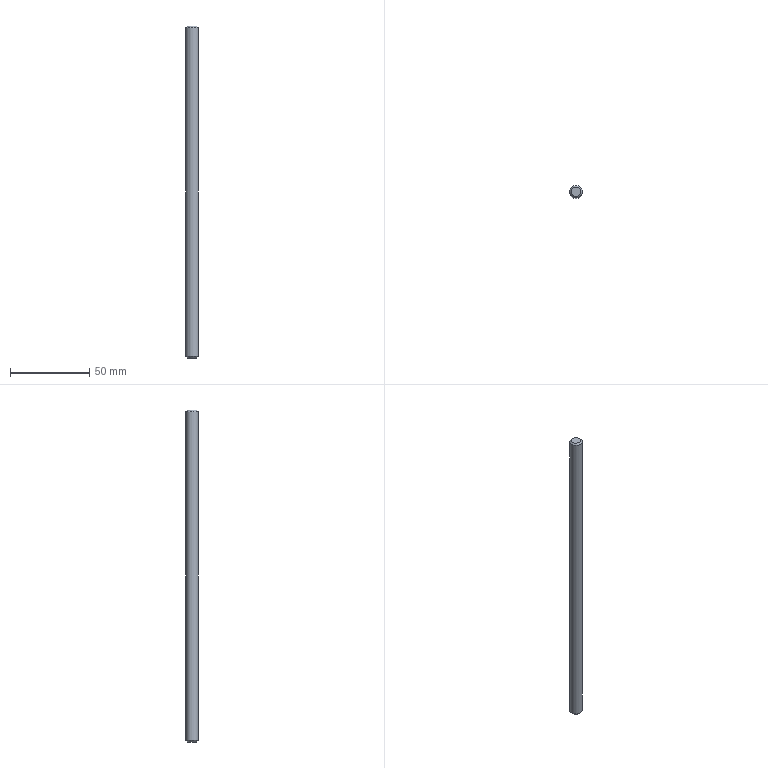Part | STEP file | Rod1 | 1 solid | 5 faces | box 8 x 8 x 210 mm | volume 10533 mm3 | cone 2 | plane 2 | cylinder 1 | commonest cylinder face diameters 8 x1
STEP:
#1=CARTESIAN_POINT('',(0.,0.,0.));
#2=DIRECTION('',(0.,0.,1.));
#3=DIRECTION('',(1.,0.,0.));
#4=AXIS2_PLACEMENT_3D('',#1,#2,#3);
#5=CARTESIAN_POINT('',(4.,0.,1.));
#6=VERTEX_POINT('',#5);
#7=CARTESIAN_POINT('',(0.,0.,1.));
#8=DIRECTION('',(0.,0.,-1.));
#9=DIRECTION('',(-1.,0.,0.));
#10=AXIS2_PLACEMENT_3D('',#7,#8,#9);
#11=CIRCLE('',#10,4.);
#12=CARTESIAN_POINT('',(0.,0.,0.5));
#13=DIRECTION('',(0.,0.,1.));
#14=DIRECTION('',(-1.,0.,0.));
#15=AXIS2_PLACEMENT_3D('',#12,#13,#14);
#16=CONICAL_SURFACE('',#15,3.5,0.7854);
#17=CARTESIAN_POINT('',(12.566,0.5));
#18=DIRECTION('',(-1.,0.));
#19=VECTOR('',#18,1.);
#20=LINE('',#17,#19);
#21=(GEOMETRIC_REPRESENTATION_CONTEXT(2)PARAMETRIC_REPRESENTATION_CONTEXT()REPRESENTATION_CONTEXT('',''));
#22=DEFINITIONAL_REPRESENTATION('',(#20),#21);
#23=PCURVE('',#16,#22);
#24=CARTESIAN_POINT('',(0.,0.,0.));
#25=DIRECTION('',(0.,0.,1.));
#26=DIRECTION('',(-1.,0.,0.));
#27=AXIS2_PLACEMENT_3D('',#24,#25,#26);
#28=CYLINDRICAL_SURFACE('',#27,4.);
#29=CARTESIAN_POINT('',(12.566,1.));
#30=DIRECTION('',(-1.,0.));
#31=VECTOR('',#30,1.);
#32=LINE('',#29,#31);
#33=(GEOMETRIC_REPRESENTATION_CONTEXT(2)PARAMETRIC_REPRESENTATION_CONTEXT()REPRESENTATION_CONTEXT('',''));
#34=DEFINITIONAL_REPRESENTATION('',(#32),#33);
#35=PCURVE('',#28,#34);
#36=SURFACE_CURVE('',#11,(#23,#35),.PCURVE_S1.);
#37=EDGE_CURVE('',#6,#6,#36,.T.);
#38=ORIENTED_EDGE('',*,*,#37,.T.);
#39=CARTESIAN_POINT('',(3.,0.,0.));
#40=VERTEX_POINT('',#39);
#41=CARTESIAN_POINT('',(3.,0.,0.));
#42=CARTESIAN_POINT('',(4.,0.,1.));
#43=B_SPLINE_CURVE_WITH_KNOTS('',1,(#41,#42),.UNSPECIFIED.,.F.,.F.,(2,2),(-0.7071,0.7071),.PIECEWISE_BEZIER_KNOTS.);
#44=CARTESIAN_POINT('',(3.142,0.));
#45=DIRECTION('',(0.,1.));
#46=VECTOR('',#45,1.);
#47=LINE('',#44,#46);
#48=(GEOMETRIC_REPRESENTATION_CONTEXT(2)PARAMETRIC_REPRESENTATION_CONTEXT()REPRESENTATION_CONTEXT('',''));
#49=DEFINITIONAL_REPRESENTATION('',(#47),#48);
#50=PCURVE('',#16,#49);
#51=CARTESIAN_POINT('',(9.425,0.));
#52=DIRECTION('',(0.,1.));
#53=VECTOR('',#52,1.);
#54=LINE('',#51,#53);
#55=(GEOMETRIC_REPRESENTATION_CONTEXT(2)PARAMETRIC_REPRESENTATION_CONTEXT()REPRESENTATION_CONTEXT('',''));
#56=DEFINITIONAL_REPRESENTATION('',(#54),#55);
#57=PCURVE('',#16,#56);
#58=SEAM_CURVE('',#43,(#50,#57),.PCURVE_S1.);
#59=EDGE_CURVE('',#40,#6,#58,.T.);
#60=ORIENTED_EDGE('',*,*,#59,.F.);
#61=CARTESIAN_POINT('',(0.,0.,0.));
#62=DIRECTION('',(0.,0.,1.));
#63=DIRECTION('',(-1.,0.,0.));
#64=AXIS2_PLACEMENT_3D('',#61,#62,#63);
#65=CIRCLE('',#64,3.);
#66=CARTESIAN_POINT('',(0.,-0.5));
#67=DIRECTION('',(1.,0.));
#68=VECTOR('',#67,1.);
#69=LINE('',#66,#68);
#70=(GEOMETRIC_REPRESENTATION_CONTEXT(2)PARAMETRIC_REPRESENTATION_CONTEXT()REPRESENTATION_CONTEXT('',''));
#71=DEFINITIONAL_REPRESENTATION('',(#69),#70);
#72=PCURVE('',#16,#71);
#73=CARTESIAN_POINT('',(0.,0.,0.));
#74=DIRECTION('',(0.,0.,1.));
#75=DIRECTION('',(1.,0.,0.));
#76=AXIS2_PLACEMENT_3D('',#73,#74,#75);
#77=PLANE('',#76);
#78=CARTESIAN_POINT('',(0.,0.));
#79=DIRECTION('',(-1.,0.));
#80=AXIS2_PLACEMENT_2D('',#78,#79);
#81=CIRCLE('',#80,3.);
#82=(GEOMETRIC_REPRESENTATION_CONTEXT(2)PARAMETRIC_REPRESENTATION_CONTEXT()REPRESENTATION_CONTEXT('',''));
#83=DEFINITIONAL_REPRESENTATION('',(#81),#82);
#84=PCURVE('',#77,#83);
#85=SURFACE_CURVE('',#65,(#72,#84),.PCURVE_S1.);
#86=EDGE_CURVE('',#40,#40,#85,.T.);
#87=ORIENTED_EDGE('',*,*,#86,.T.);
#88=ORIENTED_EDGE('',*,*,#59,.T.);
#89=EDGE_LOOP('',(#38,#60,#87,#88));
#90=FACE_BOUND('',#89,.T.);
#91=ADVANCED_FACE('',(#90),#16,.T.);
#92=CARTESIAN_POINT('',(4.,0.,209.));
#93=VERTEX_POINT('',#92);
#94=CARTESIAN_POINT('',(0.,0.,209.));
#95=DIRECTION('',(0.,0.,1.));
#96=DIRECTION('',(-1.,0.,0.));
#97=AXIS2_PLACEMENT_3D('',#94,#95,#96);
#98=CIRCLE('',#97,4.);
#99=CARTESIAN_POINT('',(0.,209.));
#100=DIRECTION('',(1.,0.));
#101=VECTOR('',#100,1.);
#102=LINE('',#99,#101);
#103=(GEOMETRIC_REPRESENTATION_CONTEXT(2)PARAMETRIC_REPRESENTATION_CONTEXT()REPRESENTATION_CONTEXT('',''));
#104=DEFINITIONAL_REPRESENTATION('',(#102),#103);
#105=PCURVE('',#28,#104);
#106=CARTESIAN_POINT('',(0.,0.,209.5));
#107=DIRECTION('',(0.,0.,-1.));
#108=DIRECTION('',(-1.,0.,0.));
#109=AXIS2_PLACEMENT_3D('',#106,#107,#108);
#110=CONICAL_SURFACE('',#109,3.5,0.7854);
#111=CARTESIAN_POINT('',(12.566,0.5));
#112=DIRECTION('',(-1.,0.));
#113=VECTOR('',#112,1.);
#114=LINE('',#111,#113);
#115=(GEOMETRIC_REPRESENTATION_CONTEXT(2)PARAMETRIC_REPRESENTATION_CONTEXT()REPRESENTATION_CONTEXT('',''));
#116=DEFINITIONAL_REPRESENTATION('',(#114),#115);
#117=PCURVE('',#110,#116);
#118=SURFACE_CURVE('',#98,(#105,#117),.PCURVE_S1.);
#119=EDGE_CURVE('',#93,#93,#118,.T.);
#120=ORIENTED_EDGE('',*,*,#119,.F.);
#121=CARTESIAN_POINT('',(4.,0.,1.));
#122=CARTESIAN_POINT('',(4.,0.,209.));
#123=B_SPLINE_CURVE_WITH_KNOTS('',1,(#121,#122),.UNSPECIFIED.,.F.,.F.,(2,2),(1.,209.),.PIECEWISE_BEZIER_KNOTS.);
#124=CARTESIAN_POINT('',(3.142,0.));
#125=DIRECTION('',(0.,1.));
#126=VECTOR('',#125,1.);
#127=LINE('',#124,#126);
#128=(GEOMETRIC_REPRESENTATION_CONTEXT(2)PARAMETRIC_REPRESENTATION_CONTEXT()REPRESENTATION_CONTEXT('',''));
#129=DEFINITIONAL_REPRESENTATION('',(#127),#128);
#130=PCURVE('',#28,#129);
#131=CARTESIAN_POINT('',(9.425,0.));
#132=DIRECTION('',(0.,1.));
#133=VECTOR('',#132,1.);
#134=LINE('',#131,#133);
#135=(GEOMETRIC_REPRESENTATION_CONTEXT(2)PARAMETRIC_REPRESENTATION_CONTEXT()REPRESENTATION_CONTEXT('',''));
#136=DEFINITIONAL_REPRESENTATION('',(#134),#135);
#137=PCURVE('',#28,#136);
#138=SEAM_CURVE('',#123,(#130,#137),.PCURVE_S1.);
#139=EDGE_CURVE('',#6,#93,#138,.T.);
#140=ORIENTED_EDGE('',*,*,#139,.F.);
#141=ORIENTED_EDGE('',*,*,#37,.F.);
#142=ORIENTED_EDGE('',*,*,#139,.T.);
#143=EDGE_LOOP('',(#120,#140,#141,#142));
#144=FACE_BOUND('',#143,.T.);
#145=ADVANCED_FACE('',(#144),#28,.T.);
#146=ORIENTED_EDGE('',*,*,#86,.F.);
#147=EDGE_LOOP('',(#146));
#148=FACE_BOUND('',#147,.T.);
#149=ADVANCED_FACE('',(#148),#77,.F.);
#150=ORIENTED_EDGE('',*,*,#119,.T.);
#151=CARTESIAN_POINT('',(3.,0.,210.));
#152=VERTEX_POINT('',#151);
#153=CARTESIAN_POINT('',(3.,0.,210.));
#154=CARTESIAN_POINT('',(4.,0.,209.));
#155=B_SPLINE_CURVE_WITH_KNOTS('',1,(#153,#154),.UNSPECIFIED.,.F.,.F.,(2,2),(-0.7071,0.7071),.PIECEWISE_BEZIER_KNOTS.);
#156=CARTESIAN_POINT('',(3.142,0.));
#157=DIRECTION('',(0.,1.));
#158=VECTOR('',#157,1.);
#159=LINE('',#156,#158);
#160=(GEOMETRIC_REPRESENTATION_CONTEXT(2)PARAMETRIC_REPRESENTATION_CONTEXT()REPRESENTATION_CONTEXT('',''));
#161=DEFINITIONAL_REPRESENTATION('',(#159),#160);
#162=PCURVE('',#110,#161);
#163=CARTESIAN_POINT('',(9.425,0.));
#164=DIRECTION('',(0.,1.));
#165=VECTOR('',#164,1.);
#166=LINE('',#163,#165);
#167=(GEOMETRIC_REPRESENTATION_CONTEXT(2)PARAMETRIC_REPRESENTATION_CONTEXT()REPRESENTATION_CONTEXT('',''));
#168=DEFINITIONAL_REPRESENTATION('',(#166),#167);
#169=PCURVE('',#110,#168);
#170=SEAM_CURVE('',#155,(#162,#169),.PCURVE_S1.);
#171=EDGE_CURVE('',#152,#93,#170,.T.);
#172=ORIENTED_EDGE('',*,*,#171,.F.);
#173=CARTESIAN_POINT('',(0.,0.,210.));
#174=DIRECTION('',(0.,0.,-1.));
#175=DIRECTION('',(-1.,0.,0.));
#176=AXIS2_PLACEMENT_3D('',#173,#174,#175);
#177=CIRCLE('',#176,3.);
#178=CARTESIAN_POINT('',(0.,-0.5));
#179=DIRECTION('',(1.,0.));
#180=VECTOR('',#179,1.);
#181=LINE('',#178,#180);
#182=(GEOMETRIC_REPRESENTATION_CONTEXT(2)PARAMETRIC_REPRESENTATION_CONTEXT()REPRESENTATION_CONTEXT('',''));
#183=DEFINITIONAL_REPRESENTATION('',(#181),#182);
#184=PCURVE('',#110,#183);
#185=CARTESIAN_POINT('',(0.,0.,210.));
#186=DIRECTION('',(0.,0.,1.));
#187=DIRECTION('',(1.,0.,0.));
#188=AXIS2_PLACEMENT_3D('',#185,#186,#187);
#189=PLANE('',#188);
#190=CARTESIAN_POINT('',(-3.,0.));
#191=CARTESIAN_POINT('',(-3.,5.196));
#192=CARTESIAN_POINT('',(1.5,2.598));
#193=CARTESIAN_POINT('',(6.,0.));
#194=CARTESIAN_POINT('',(1.5,-2.598));
#195=CARTESIAN_POINT('',(-3.,-5.196));
#196=CARTESIAN_POINT('',(-3.,0.));
#197=(BOUNDED_CURVE()B_SPLINE_CURVE(2,(#190,#191,#192,#193,#194,#195,#196),.UNSPECIFIED.,.T.,.F.)B_SPLINE_CURVE_WITH_KNOTS((1,2,2,2,2,1),(-2.094,0.,2.094,4.189,6.283,8.378),.UNSPECIFIED.)CURVE()GEOMETRIC_REPRESENTATION_ITEM()RATIONAL_B_SPLINE_CURVE((1.,0.5,1.,0.5,1.,0.5,1.))REPRESENTATION_ITEM(''));
#198=(GEOMETRIC_REPRESENTATION_CONTEXT(2)PARAMETRIC_REPRESENTATION_CONTEXT()REPRESENTATION_CONTEXT('',''));
#199=DEFINITIONAL_REPRESENTATION('',(#197),#198);
#200=PCURVE('',#189,#199);
#201=SURFACE_CURVE('',#177,(#184,#200),.PCURVE_S1.);
#202=EDGE_CURVE('',#152,#152,#201,.T.);
#203=ORIENTED_EDGE('',*,*,#202,.T.);
#204=ORIENTED_EDGE('',*,*,#171,.T.);
#205=EDGE_LOOP('',(#150,#172,#203,#204));
#206=FACE_BOUND('',#205,.T.);
#207=ADVANCED_FACE('',(#206),#110,.T.);
#208=ORIENTED_EDGE('',*,*,#202,.F.);
#209=EDGE_LOOP('',(#208));
#210=FACE_BOUND('',#209,.T.);
#211=ADVANCED_FACE('',(#210),#189,.T.);
#212=CLOSED_SHELL('',(#91,#145,#149,#207,#211));
#213=MANIFOLD_SOLID_BREP('',#212);
#214=(LENGTH_UNIT()NAMED_UNIT(*)SI_UNIT(.MILLI.,.METRE.));
#215=UNCERTAINTY_MEASURE_WITH_UNIT(LENGTH_MEASURE(0.00001),#214,'','');
#216=(NAMED_UNIT(*)PLANE_ANGLE_UNIT()SI_UNIT($,.RADIAN.));
#217=(NAMED_UNIT(*)SI_UNIT($,.STERADIAN.)SOLID_ANGLE_UNIT());
#218=(GEOMETRIC_REPRESENTATION_CONTEXT(3)GLOBAL_UNCERTAINTY_ASSIGNED_CONTEXT((#215))GLOBAL_UNIT_ASSIGNED_CONTEXT((#214,#216,#217))REPRESENTATION_CONTEXT('',''));
#219=ADVANCED_BREP_SHAPE_REPRESENTATION('',(#4,#213),#218);